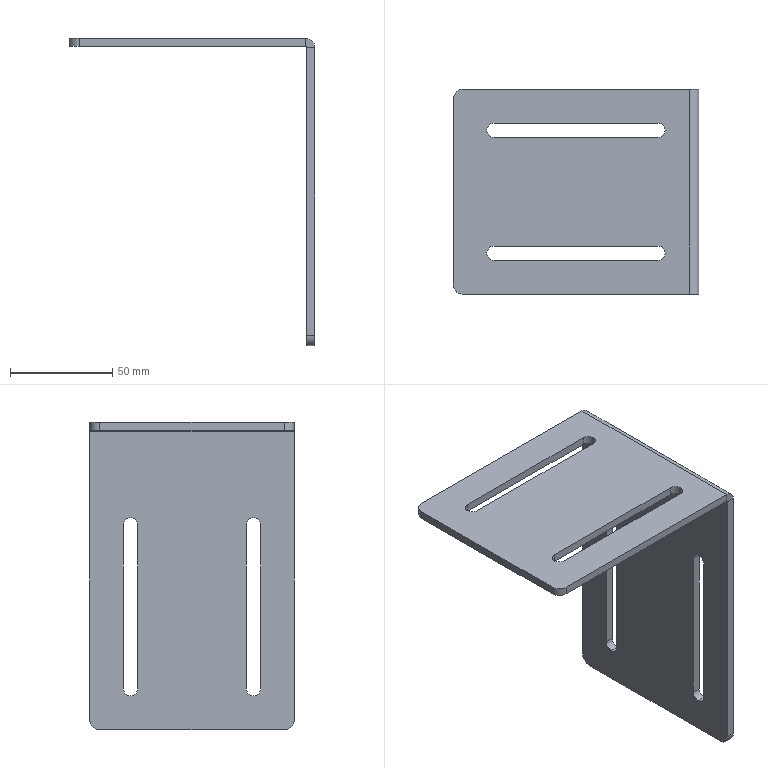Part | SolidWorks | features ICE 2, EdgeFlange 1, Fillet 1, FlatPattern 1, SMBaseFlange 1, SheetMetal 1 | 1 solid | 38 faces | box 120 x 100 x 150 mm | volume 96309 mm3 | plane 20 | cylinder 18 | commonest cylinder face diameters 7 x12 10 x4 1 x1 9 x1
STEP:
#1=CARTESIAN_POINT('',(56.,33.5,-130.));
#2=VERTEX_POINT('',#1);
#3=CARTESIAN_POINT('',(56.,30.,-133.5));
#4=VERTEX_POINT('',#3);
#5=CARTESIAN_POINT('',(56.,30.,-130.));
#6=DIRECTION('',(-1.,0.,0.));
#7=DIRECTION('',(0.,0.,-1.));
#8=AXIS2_PLACEMENT_3D('',#5,#6,#7);
#9=CIRCLE('',#8,3.5);
#10=EDGE_CURVE('',#2,#4,#9,.T.);
#11=ORIENTED_EDGE('',*,*,#10,.T.);
#12=CARTESIAN_POINT('',(60.,30.,-133.5));
#13=VERTEX_POINT('',#12);
#14=CARTESIAN_POINT('',(-60.,30.,-133.5));
#15=DIRECTION('',(1.,0.,0.));
#16=VECTOR('',#15,1000.);
#17=LINE('',#14,#16);
#18=EDGE_CURVE('',#4,#13,#17,.T.);
#19=ORIENTED_EDGE('',*,*,#18,.T.);
#20=CARTESIAN_POINT('',(60.,33.5,-130.));
#21=VERTEX_POINT('',#20);
#22=CARTESIAN_POINT('',(60.,30.,-130.));
#23=DIRECTION('',(-1.,0.,0.));
#24=DIRECTION('',(0.,0.,-1.));
#25=AXIS2_PLACEMENT_3D('',#22,#23,#24);
#26=CIRCLE('',#25,3.5);
#27=EDGE_CURVE('',#21,#13,#26,.T.);
#28=ORIENTED_EDGE('',*,*,#27,.F.);
#29=CARTESIAN_POINT('',(-60.,33.5,-130.));
#30=DIRECTION('',(1.,0.,0.));
#31=VECTOR('',#30,1000.);
#32=LINE('',#29,#31);
#33=EDGE_CURVE('',#2,#21,#32,.T.);
#34=ORIENTED_EDGE('',*,*,#33,.F.);
#35=EDGE_LOOP('',(#11,#19,#28,#34));
#36=FACE_OUTER_BOUND('',#35,.T.);
#37=CARTESIAN_POINT('',(-60.,30.,-130.));
#38=DIRECTION('',(1.,0.,0.));
#39=DIRECTION('',(0.,0.,-1.));
#40=AXIS2_PLACEMENT_3D('',#37,#38,#39);
#41=CYLINDRICAL_SURFACE('',#40,3.5);
#42=ADVANCED_FACE('',(#36),#41,.F.);
#43=CARTESIAN_POINT('',(56.,-26.5,-130.));
#44=VERTEX_POINT('',#43);
#45=CARTESIAN_POINT('',(56.,-30.,-133.5));
#46=VERTEX_POINT('',#45);
#47=CARTESIAN_POINT('',(56.,-30.,-130.));
#48=DIRECTION('',(-1.,0.,0.));
#49=DIRECTION('',(0.,0.,-1.));
#50=AXIS2_PLACEMENT_3D('',#47,#48,#49);
#51=CIRCLE('',#50,3.5);
#52=EDGE_CURVE('',#44,#46,#51,.T.);
#53=ORIENTED_EDGE('',*,*,#52,.T.);
#54=CARTESIAN_POINT('',(60.,-30.,-133.5));
#55=VERTEX_POINT('',#54);
#56=CARTESIAN_POINT('',(-60.,-30.,-133.5));
#57=DIRECTION('',(1.,0.,0.));
#58=VECTOR('',#57,1000.);
#59=LINE('',#56,#58);
#60=EDGE_CURVE('',#46,#55,#59,.T.);
#61=ORIENTED_EDGE('',*,*,#60,.T.);
#62=CARTESIAN_POINT('',(60.,-26.5,-130.));
#63=VERTEX_POINT('',#62);
#64=CARTESIAN_POINT('',(60.,-30.,-130.));
#65=DIRECTION('',(-1.,0.,0.));
#66=DIRECTION('',(0.,0.,-1.));
#67=AXIS2_PLACEMENT_3D('',#64,#65,#66);
#68=CIRCLE('',#67,3.5);
#69=EDGE_CURVE('',#63,#55,#68,.T.);
#70=ORIENTED_EDGE('',*,*,#69,.F.);
#71=CARTESIAN_POINT('',(-60.,-26.5,-130.));
#72=DIRECTION('',(1.,0.,0.));
#73=VECTOR('',#72,1000.);
#74=LINE('',#71,#73);
#75=EDGE_CURVE('',#44,#63,#74,.T.);
#76=ORIENTED_EDGE('',*,*,#75,.F.);
#77=EDGE_LOOP('',(#53,#61,#70,#76));
#78=FACE_OUTER_BOUND('',#77,.T.);
#79=CARTESIAN_POINT('',(-60.,-30.,-130.));
#80=DIRECTION('',(1.,0.,0.));
#81=DIRECTION('',(0.,0.,-1.));
#82=AXIS2_PLACEMENT_3D('',#79,#80,#81);
#83=CYLINDRICAL_SURFACE('',#82,3.5);
#84=ADVANCED_FACE('',(#78),#83,.F.);
#85=CARTESIAN_POINT('',(40.,33.5,-4.));
#86=VERTEX_POINT('',#85);
#87=CARTESIAN_POINT('',(43.5,30.,-4.));
#88=VERTEX_POINT('',#87);
#89=CARTESIAN_POINT('',(40.,30.,-4.));
#90=DIRECTION('',(0.,0.,-1.));
#91=DIRECTION('',(1.,0.,0.));
#92=AXIS2_PLACEMENT_3D('',#89,#90,#91);
#93=CIRCLE('',#92,3.5);
#94=EDGE_CURVE('',#86,#88,#93,.T.);
#95=ORIENTED_EDGE('',*,*,#94,.T.);
#96=CARTESIAN_POINT('',(43.5,30.,0.));
#97=VERTEX_POINT('',#96);
#98=CARTESIAN_POINT('',(43.5,30.,-150.001));
#99=DIRECTION('',(0.,0.,1.));
#100=VECTOR('',#99,1000.);
#101=LINE('',#98,#100);
#102=EDGE_CURVE('',#88,#97,#101,.T.);
#103=ORIENTED_EDGE('',*,*,#102,.T.);
#104=CARTESIAN_POINT('',(40.,33.5,0.));
#105=VERTEX_POINT('',#104);
#106=CARTESIAN_POINT('',(40.,30.,0.));
#107=DIRECTION('',(0.,0.,1.));
#108=DIRECTION('',(1.,0.,0.));
#109=AXIS2_PLACEMENT_3D('',#106,#107,#108);
#110=CIRCLE('',#109,3.5);
#111=EDGE_CURVE('',#97,#105,#110,.T.);
#112=ORIENTED_EDGE('',*,*,#111,.T.);
#113=CARTESIAN_POINT('',(40.,33.5,-150.001));
#114=DIRECTION('',(0.,0.,1.));
#115=VECTOR('',#114,1000.);
#116=LINE('',#113,#115);
#117=EDGE_CURVE('',#86,#105,#116,.T.);
#118=ORIENTED_EDGE('',*,*,#117,.F.);
#119=EDGE_LOOP('',(#95,#103,#112,#118));
#120=FACE_OUTER_BOUND('',#119,.T.);
#121=CARTESIAN_POINT('',(40.,30.,-150.001));
#122=DIRECTION('',(0.,0.,1.));
#123=DIRECTION('',(1.,0.,0.));
#124=AXIS2_PLACEMENT_3D('',#121,#122,#123);
#125=CYLINDRICAL_SURFACE('',#124,3.5);
#126=ADVANCED_FACE('',(#120),#125,.F.);
#127=CARTESIAN_POINT('',(40.,-26.5,-4.));
#128=VERTEX_POINT('',#127);
#129=CARTESIAN_POINT('',(43.5,-30.,-4.));
#130=VERTEX_POINT('',#129);
#131=CARTESIAN_POINT('',(40.,-30.,-4.));
#132=DIRECTION('',(0.,0.,-1.));
#133=DIRECTION('',(1.,0.,0.));
#134=AXIS2_PLACEMENT_3D('',#131,#132,#133);
#135=CIRCLE('',#134,3.5);
#136=EDGE_CURVE('',#128,#130,#135,.T.);
#137=ORIENTED_EDGE('',*,*,#136,.T.);
#138=CARTESIAN_POINT('',(43.5,-30.,0.));
#139=VERTEX_POINT('',#138);
#140=CARTESIAN_POINT('',(43.5,-30.,-150.001));
#141=DIRECTION('',(0.,0.,1.));
#142=VECTOR('',#141,1000.);
#143=LINE('',#140,#142);
#144=EDGE_CURVE('',#130,#139,#143,.T.);
#145=ORIENTED_EDGE('',*,*,#144,.T.);
#146=CARTESIAN_POINT('',(40.,-26.5,0.));
#147=VERTEX_POINT('',#146);
#148=CARTESIAN_POINT('',(40.,-30.,0.));
#149=DIRECTION('',(0.,0.,1.));
#150=DIRECTION('',(1.,0.,0.));
#151=AXIS2_PLACEMENT_3D('',#148,#149,#150);
#152=CIRCLE('',#151,3.5);
#153=EDGE_CURVE('',#139,#147,#152,.T.);
#154=ORIENTED_EDGE('',*,*,#153,.T.);
#155=CARTESIAN_POINT('',(40.,-26.5,-150.001));
#156=DIRECTION('',(0.,0.,1.));
#157=VECTOR('',#156,1000.);
#158=LINE('',#155,#157);
#159=EDGE_CURVE('',#128,#147,#158,.T.);
#160=ORIENTED_EDGE('',*,*,#159,.F.);
#161=EDGE_LOOP('',(#137,#145,#154,#160));
#162=FACE_OUTER_BOUND('',#161,.T.);
#163=CARTESIAN_POINT('',(40.,-30.,-150.001));
#164=DIRECTION('',(0.,0.,1.));
#165=DIRECTION('',(1.,0.,0.));
#166=AXIS2_PLACEMENT_3D('',#163,#164,#165);
#167=CYLINDRICAL_SURFACE('',#166,3.5);
#168=ADVANCED_FACE('',(#162),#167,.F.);
#169=CARTESIAN_POINT('',(60.,-50.,-145.));
#170=VERTEX_POINT('',#169);
#171=CARTESIAN_POINT('',(60.,-50.,-4.5));
#172=VERTEX_POINT('',#171);
#173=CARTESIAN_POINT('',(60.,-50.,-4.));
#174=DIRECTION('',(0.,0.,1.));
#175=VECTOR('',#174,1000.);
#176=LINE('',#173,#175);
#177=EDGE_CURVE('',#170,#172,#176,.T.);
#178=ORIENTED_EDGE('',*,*,#177,.F.);
#179=CARTESIAN_POINT('',(60.,-45.,-150.));
#180=VERTEX_POINT('',#179);
#181=CARTESIAN_POINT('',(60.,-45.,-145.));
#182=DIRECTION('',(1.,0.,0.));
#183=DIRECTION('',(0.,0.,-1.));
#184=AXIS2_PLACEMENT_3D('',#181,#182,#183);
#185=CIRCLE('',#184,5.);
#186=EDGE_CURVE('',#170,#180,#185,.T.);
#187=ORIENTED_EDGE('',*,*,#186,.T.);
#188=CARTESIAN_POINT('',(60.,45.,-150.));
#189=VERTEX_POINT('',#188);
#190=CARTESIAN_POINT('',(60.,-50.,-150.));
#191=DIRECTION('',(0.,-1.,0.));
#192=VECTOR('',#191,1000.);
#193=LINE('',#190,#192);
#194=EDGE_CURVE('',#189,#180,#193,.T.);
#195=ORIENTED_EDGE('',*,*,#194,.F.);
#196=CARTESIAN_POINT('',(60.,50.,-145.));
#197=VERTEX_POINT('',#196);
#198=CARTESIAN_POINT('',(60.,45.,-145.));
#199=DIRECTION('',(1.,0.,0.));
#200=DIRECTION('',(0.,0.,-1.));
#201=AXIS2_PLACEMENT_3D('',#198,#199,#200);
#202=CIRCLE('',#201,5.);
#203=EDGE_CURVE('',#189,#197,#202,.T.);
#204=ORIENTED_EDGE('',*,*,#203,.T.);
#205=CARTESIAN_POINT('',(60.,50.,-4.5));
#206=VERTEX_POINT('',#205);
#207=CARTESIAN_POINT('',(60.,50.,-150.));
#208=DIRECTION('',(0.,0.,-1.));
#209=VECTOR('',#208,1000.);
#210=LINE('',#207,#209);
#211=EDGE_CURVE('',#206,#197,#210,.T.);
#212=ORIENTED_EDGE('',*,*,#211,.F.);
#213=CARTESIAN_POINT('',(60.,0.,-4.5));
#214=DIRECTION('',(0.,-1.,0.));
#215=VECTOR('',#214,1000.);
#216=LINE('',#213,#215);
#217=EDGE_CURVE('',#206,#172,#216,.T.);
#218=ORIENTED_EDGE('',*,*,#217,.T.);
#219=EDGE_LOOP('',(#178,#187,#195,#204,#212,#218));
#220=FACE_OUTER_BOUND('',#219,.T.);
#221=CARTESIAN_POINT('',(60.,-26.5,-50.));
#222=VERTEX_POINT('',#221);
#223=CARTESIAN_POINT('',(60.,-26.5,-130.));
#224=DIRECTION('',(0.,0.,-1.));
#225=VECTOR('',#224,1000.);
#226=LINE('',#223,#225);
#227=EDGE_CURVE('',#222,#63,#226,.T.);
#228=ORIENTED_EDGE('',*,*,#227,.T.);
#229=ORIENTED_EDGE('',*,*,#69,.T.);
#230=CARTESIAN_POINT('',(60.,-33.5,-130.));
#231=VERTEX_POINT('',#230);
#232=CARTESIAN_POINT('',(60.,-30.,-130.));
#233=DIRECTION('',(-1.,0.,0.));
#234=DIRECTION('',(0.,0.,-1.));
#235=AXIS2_PLACEMENT_3D('',#232,#233,#234);
#236=CIRCLE('',#235,3.5);
#237=EDGE_CURVE('',#55,#231,#236,.T.);
#238=ORIENTED_EDGE('',*,*,#237,.T.);
#239=CARTESIAN_POINT('',(60.,-33.5,-50.));
#240=VERTEX_POINT('',#239);
#241=CARTESIAN_POINT('',(60.,-33.5,-130.));
#242=DIRECTION('',(0.,0.,1.));
#243=VECTOR('',#242,1000.);
#244=LINE('',#241,#243);
#245=EDGE_CURVE('',#231,#240,#244,.T.);
#246=ORIENTED_EDGE('',*,*,#245,.T.);
#247=CARTESIAN_POINT('',(60.,-30.,-50.));
#248=DIRECTION('',(-1.,0.,0.));
#249=DIRECTION('',(0.,0.,-1.));
#250=AXIS2_PLACEMENT_3D('',#247,#248,#249);
#251=CIRCLE('',#250,3.5);
#252=EDGE_CURVE('',#240,#222,#251,.T.);
#253=ORIENTED_EDGE('',*,*,#252,.T.);
#254=EDGE_LOOP('',(#228,#229,#238,#246,#253));
#255=FACE_BOUND('',#254,.T.);
#256=CARTESIAN_POINT('',(60.,33.5,-50.));
#257=VERTEX_POINT('',#256);
#258=CARTESIAN_POINT('',(60.,33.5,-130.));
#259=DIRECTION('',(0.,0.,-1.));
#260=VECTOR('',#259,1000.);
#261=LINE('',#258,#260);
#262=EDGE_CURVE('',#257,#21,#261,.T.);
#263=ORIENTED_EDGE('',*,*,#262,.T.);
#264=ORIENTED_EDGE('',*,*,#27,.T.);
#265=CARTESIAN_POINT('',(60.,26.5,-130.));
#266=VERTEX_POINT('',#265);
#267=CARTESIAN_POINT('',(60.,30.,-130.));
#268=DIRECTION('',(-1.,0.,0.));
#269=DIRECTION('',(0.,0.,-1.));
#270=AXIS2_PLACEMENT_3D('',#267,#268,#269);
#271=CIRCLE('',#270,3.5);
#272=EDGE_CURVE('',#13,#266,#271,.T.);
#273=ORIENTED_EDGE('',*,*,#272,.T.);
#274=CARTESIAN_POINT('',(60.,26.5,-50.));
#275=VERTEX_POINT('',#274);
#276=CARTESIAN_POINT('',(60.,26.5,-130.));
#277=DIRECTION('',(0.,0.,1.));
#278=VECTOR('',#277,1000.);
#279=LINE('',#276,#278);
#280=EDGE_CURVE('',#266,#275,#279,.T.);
#281=ORIENTED_EDGE('',*,*,#280,.T.);
#282=CARTESIAN_POINT('',(60.,30.,-50.));
#283=DIRECTION('',(-1.,0.,0.));
#284=DIRECTION('',(0.,0.,-1.));
#285=AXIS2_PLACEMENT_3D('',#282,#283,#284);
#286=CIRCLE('',#285,3.5);
#287=EDGE_CURVE('',#275,#257,#286,.T.);
#288=ORIENTED_EDGE('',*,*,#287,.T.);
#289=EDGE_LOOP('',(#263,#264,#273,#281,#288));
#290=FACE_BOUND('',#289,.T.);
#291=CARTESIAN_POINT('',(60.,0.,0.));
#292=DIRECTION('',(1.,0.,0.));
#293=DIRECTION('',(0.,0.,-1.));
#294=AXIS2_PLACEMENT_3D('',#291,#292,#293);
#295=PLANE('',#294);
#296=ADVANCED_FACE('',(#220,#255,#290),#295,.T.);
#297=ORIENTED_EDGE('',*,*,#52,.F.);
#298=CARTESIAN_POINT('',(56.,-26.5,-50.));
#299=VERTEX_POINT('',#298);
#300=CARTESIAN_POINT('',(56.,-26.5,0.));
#301=DIRECTION('',(0.,0.,-1.));
#302=VECTOR('',#301,1000.);
#303=LINE('',#300,#302);
#304=EDGE_CURVE('',#299,#44,#303,.T.);
#305=ORIENTED_EDGE('',*,*,#304,.F.);
#306=CARTESIAN_POINT('',(56.,-33.5,-50.));
#307=VERTEX_POINT('',#306);
#308=CARTESIAN_POINT('',(56.,-30.,-50.));
#309=DIRECTION('',(-1.,0.,0.));
#310=DIRECTION('',(0.,0.,-1.));
#311=AXIS2_PLACEMENT_3D('',#308,#309,#310);
#312=CIRCLE('',#311,3.5);
#313=EDGE_CURVE('',#307,#299,#312,.T.);
#314=ORIENTED_EDGE('',*,*,#313,.F.);
#315=CARTESIAN_POINT('',(56.,-33.5,-130.));
#316=VERTEX_POINT('',#315);
#317=CARTESIAN_POINT('',(56.,-33.5,0.));
#318=DIRECTION('',(0.,0.,1.));
#319=VECTOR('',#318,1000.);
#320=LINE('',#317,#319);
#321=EDGE_CURVE('',#316,#307,#320,.T.);
#322=ORIENTED_EDGE('',*,*,#321,.F.);
#323=CARTESIAN_POINT('',(56.,-30.,-130.));
#324=DIRECTION('',(-1.,0.,0.));
#325=DIRECTION('',(0.,0.,-1.));
#326=AXIS2_PLACEMENT_3D('',#323,#324,#325);
#327=CIRCLE('',#326,3.5);
#328=EDGE_CURVE('',#46,#316,#327,.T.);
#329=ORIENTED_EDGE('',*,*,#328,.F.);
#330=EDGE_LOOP('',(#297,#305,#314,#322,#329));
#331=FACE_BOUND('',#330,.T.);
#332=CARTESIAN_POINT('',(56.,45.,-150.));
#333=VERTEX_POINT('',#332);
#334=CARTESIAN_POINT('',(56.,-45.,-150.));
#335=VERTEX_POINT('',#334);
#336=CARTESIAN_POINT('',(56.,0.,-150.));
#337=DIRECTION('',(0.,-1.,0.));
#338=VECTOR('',#337,1000.);
#339=LINE('',#336,#338);
#340=EDGE_CURVE('',#333,#335,#339,.T.);
#341=ORIENTED_EDGE('',*,*,#340,.T.);
#342=CARTESIAN_POINT('',(56.,-50.,-145.));
#343=VERTEX_POINT('',#342);
#344=CARTESIAN_POINT('',(56.,-45.,-145.));
#345=DIRECTION('',(-1.,0.,0.));
#346=DIRECTION('',(0.,0.,-1.));
#347=AXIS2_PLACEMENT_3D('',#344,#345,#346);
#348=CIRCLE('',#347,5.);
#349=EDGE_CURVE('',#335,#343,#348,.T.);
#350=ORIENTED_EDGE('',*,*,#349,.T.);
#351=CARTESIAN_POINT('',(56.,-50.,-4.5));
#352=VERTEX_POINT('',#351);
#353=CARTESIAN_POINT('',(56.,-50.,0.));
#354=DIRECTION('',(0.,0.,1.));
#355=VECTOR('',#354,1000.);
#356=LINE('',#353,#355);
#357=EDGE_CURVE('',#343,#352,#356,.T.);
#358=ORIENTED_EDGE('',*,*,#357,.T.);
#359=CARTESIAN_POINT('',(56.,50.,-4.5));
#360=VERTEX_POINT('',#359);
#361=CARTESIAN_POINT('',(56.,50.,-4.5));
#362=DIRECTION('',(0.,-1.,0.));
#363=VECTOR('',#362,1000.);
#364=LINE('',#361,#363);
#365=EDGE_CURVE('',#360,#352,#364,.T.);
#366=ORIENTED_EDGE('',*,*,#365,.F.);
#367=CARTESIAN_POINT('',(56.,50.,-145.));
#368=VERTEX_POINT('',#367);
#369=CARTESIAN_POINT('',(56.,50.,0.));
#370=DIRECTION('',(0.,0.,-1.));
#371=VECTOR('',#370,1000.);
#372=LINE('',#369,#371);
#373=EDGE_CURVE('',#360,#368,#372,.T.);
#374=ORIENTED_EDGE('',*,*,#373,.T.);
#375=CARTESIAN_POINT('',(56.,45.,-145.));
#376=DIRECTION('',(-1.,0.,0.));
#377=DIRECTION('',(0.,0.,-1.));
#378=AXIS2_PLACEMENT_3D('',#375,#376,#377);
#379=CIRCLE('',#378,5.);
#380=EDGE_CURVE('',#368,#333,#379,.T.);
#381=ORIENTED_EDGE('',*,*,#380,.T.);
#382=EDGE_LOOP('',(#341,#350,#358,#366,#374,#381));
#383=FACE_OUTER_BOUND('',#382,.T.);
#384=ORIENTED_EDGE('',*,*,#10,.F.);
#385=CARTESIAN_POINT('',(56.,33.5,-50.));
#386=VERTEX_POINT('',#385);
#387=CARTESIAN_POINT('',(56.,33.5,0.));
#388=DIRECTION('',(0.,0.,-1.));
#389=VECTOR('',#388,1000.);
#390=LINE('',#387,#389);
#391=EDGE_CURVE('',#386,#2,#390,.T.);
#392=ORIENTED_EDGE('',*,*,#391,.F.);
#393=CARTESIAN_POINT('',(56.,26.5,-50.));
#394=VERTEX_POINT('',#393);
#395=CARTESIAN_POINT('',(56.,30.,-50.));
#396=DIRECTION('',(-1.,0.,0.));
#397=DIRECTION('',(0.,0.,-1.));
#398=AXIS2_PLACEMENT_3D('',#395,#396,#397);
#399=CIRCLE('',#398,3.5);
#400=EDGE_CURVE('',#394,#386,#399,.T.);
#401=ORIENTED_EDGE('',*,*,#400,.F.);
#402=CARTESIAN_POINT('',(56.,26.5,-130.));
#403=VERTEX_POINT('',#402);
#404=CARTESIAN_POINT('',(56.,26.5,0.));
#405=DIRECTION('',(0.,0.,1.));
#406=VECTOR('',#405,1000.);
#407=LINE('',#404,#406);
#408=EDGE_CURVE('',#403,#394,#407,.T.);
#409=ORIENTED_EDGE('',*,*,#408,.F.);
#410=CARTESIAN_POINT('',(56.,30.,-130.));
#411=DIRECTION('',(-1.,0.,0.));
#412=DIRECTION('',(0.,0.,-1.));
#413=AXIS2_PLACEMENT_3D('',#410,#411,#412);
#414=CIRCLE('',#413,3.5);
#415=EDGE_CURVE('',#4,#403,#414,.T.);
#416=ORIENTED_EDGE('',*,*,#415,.F.);
#417=EDGE_LOOP('',(#384,#392,#401,#409,#416));
#418=FACE_BOUND('',#417,.T.);
#419=CARTESIAN_POINT('',(56.,0.,0.));
#420=DIRECTION('',(1.,0.,0.));
#421=DIRECTION('',(0.,0.,-1.));
#422=AXIS2_PLACEMENT_3D('',#419,#420,#421);
#423=PLANE('',#422);
#424=ADVANCED_FACE('',(#331,#383,#418),#423,.F.);
#425=CARTESIAN_POINT('',(-55.,-50.,0.));
#426=VERTEX_POINT('',#425);
#427=CARTESIAN_POINT('',(55.5,-50.,0.));
#428=VERTEX_POINT('',#427);
#429=CARTESIAN_POINT('',(60.,-50.,0.));
#430=DIRECTION('',(1.,0.,0.));
#431=VECTOR('',#430,1000.);
#432=LINE('',#429,#431);
#433=EDGE_CURVE('',#426,#428,#432,.T.);
#434=ORIENTED_EDGE('',*,*,#433,.F.);
#435=CARTESIAN_POINT('',(-55.,-50.,-4.));
#436=VERTEX_POINT('',#435);
#437=CARTESIAN_POINT('',(-55.,-50.,-4.));
#438=DIRECTION('',(0.,0.,-1.));
#439=VECTOR('',#438,1000.);
#440=LINE('',#437,#439);
#441=EDGE_CURVE('',#426,#436,#440,.T.);
#442=ORIENTED_EDGE('',*,*,#441,.T.);
#443=CARTESIAN_POINT('',(55.5,-50.,-4.));
#444=VERTEX_POINT('',#443);
#445=CARTESIAN_POINT('',(60.,-50.,-4.));
#446=DIRECTION('',(1.,0.,0.));
#447=VECTOR('',#446,1000.);
#448=LINE('',#445,#447);
#449=EDGE_CURVE('',#436,#444,#448,.T.);
#450=ORIENTED_EDGE('',*,*,#449,.T.);
#451=CARTESIAN_POINT('',(55.5,-50.,-4.));
#452=DIRECTION('',(0.,0.,1.));
#453=VECTOR('',#452,1000.);
#454=LINE('',#451,#453);
#455=EDGE_CURVE('',#444,#428,#454,.T.);
#456=ORIENTED_EDGE('',*,*,#455,.T.);
#457=EDGE_LOOP('',(#434,#442,#450,#456));
#458=FACE_OUTER_BOUND('',#457,.T.);
#459=CARTESIAN_POINT('',(60.,-50.,-4.));
#460=DIRECTION('',(0.,-1.,0.));
#461=DIRECTION('',(1.,0.,0.));
#462=AXIS2_PLACEMENT_3D('',#459,#460,#461);
#463=PLANE('',#462);
#464=ADVANCED_FACE('',(#458),#463,.T.);
#465=CARTESIAN_POINT('',(-40.,33.5,-4.));
#466=VERTEX_POINT('',#465);
#467=CARTESIAN_POINT('',(-40.,33.5,-4.));
#468=DIRECTION('',(1.,0.,0.));
#469=VECTOR('',#468,1000.);
#470=LINE('',#467,#469);
#471=EDGE_CURVE('',#466,#86,#470,.T.);
#472=ORIENTED_EDGE('',*,*,#471,.F.);
#473=CARTESIAN_POINT('',(-40.,26.5,-4.));
#474=VERTEX_POINT('',#473);
#475=CARTESIAN_POINT('',(-40.,30.,-4.));
#476=DIRECTION('',(0.,0.,-1.));
#477=DIRECTION('',(1.,0.,0.));
#478=AXIS2_PLACEMENT_3D('',#475,#476,#477);
#479=CIRCLE('',#478,3.5);
#480=EDGE_CURVE('',#474,#466,#479,.T.);
#481=ORIENTED_EDGE('',*,*,#480,.F.);
#482=CARTESIAN_POINT('',(40.,26.5,-4.));
#483=VERTEX_POINT('',#482);
#484=CARTESIAN_POINT('',(-40.,26.5,-4.));
#485=DIRECTION('',(-1.,0.,0.));
#486=VECTOR('',#485,1000.);
#487=LINE('',#484,#486);
#488=EDGE_CURVE('',#483,#474,#487,.T.);
#489=ORIENTED_EDGE('',*,*,#488,.F.);
#490=CARTESIAN_POINT('',(40.,30.,-4.));
#491=DIRECTION('',(0.,0.,-1.));
#492=DIRECTION('',(1.,0.,0.));
#493=AXIS2_PLACEMENT_3D('',#490,#491,#492);
#494=CIRCLE('',#493,3.5);
#495=EDGE_CURVE('',#88,#483,#494,.T.);
#496=ORIENTED_EDGE('',*,*,#495,.F.);
#497=ORIENTED_EDGE('',*,*,#94,.F.);
#498=EDGE_LOOP('',(#472,#481,#489,#496,#497));
#499=FACE_BOUND('',#498,.T.);
#500=CARTESIAN_POINT('',(-40.,-26.5,-4.));
#501=VERTEX_POINT('',#500);
#502=CARTESIAN_POINT('',(-40.,-26.5,-4.));
#503=DIRECTION('',(1.,0.,0.));
#504=VECTOR('',#503,1000.);
#505=LINE('',#502,#504);
#506=EDGE_CURVE('',#501,#128,#505,.T.);
#507=ORIENTED_EDGE('',*,*,#506,.F.);
#508=CARTESIAN_POINT('',(-40.,-33.5,-4.));
#509=VERTEX_POINT('',#508);
#510=CARTESIAN_POINT('',(-40.,-30.,-4.));
#511=DIRECTION('',(0.,0.,-1.));
#512=DIRECTION('',(1.,0.,0.));
#513=AXIS2_PLACEMENT_3D('',#510,#511,#512);
#514=CIRCLE('',#513,3.5);
#515=EDGE_CURVE('',#509,#501,#514,.T.);
#516=ORIENTED_EDGE('',*,*,#515,.F.);
#517=CARTESIAN_POINT('',(40.,-33.5,-4.));
#518=VERTEX_POINT('',#517);
#519=CARTESIAN_POINT('',(-40.,-33.5,-4.));
#520=DIRECTION('',(-1.,0.,0.));
#521=VECTOR('',#520,1000.);
#522=LINE('',#519,#521);
#523=EDGE_CURVE('',#518,#509,#522,.T.);
#524=ORIENTED_EDGE('',*,*,#523,.F.);
#525=CARTESIAN_POINT('',(40.,-30.,-4.));
#526=DIRECTION('',(0.,0.,-1.));
#527=DIRECTION('',(1.,0.,0.));
#528=AXIS2_PLACEMENT_3D('',#525,#526,#527);
#529=CIRCLE('',#528,3.5);
#530=EDGE_CURVE('',#130,#518,#529,.T.);
#531=ORIENTED_EDGE('',*,*,#530,.F.);
#532=ORIENTED_EDGE('',*,*,#136,.F.);
#533=EDGE_LOOP('',(#507,#516,#524,#531,#532));
#534=FACE_BOUND('',#533,.T.);
#535=ORIENTED_EDGE('',*,*,#449,.F.);
#536=CARTESIAN_POINT('',(-60.,-45.,-4.));
#537=VERTEX_POINT('',#536);
#538=CARTESIAN_POINT('',(-55.,-45.,-4.));
#539=DIRECTION('',(0.,0.,-1.));
#540=DIRECTION('',(1.,0.,0.));
#541=AXIS2_PLACEMENT_3D('',#538,#539,#540);
#542=CIRCLE('',#541,5.);
#543=EDGE_CURVE('',#436,#537,#542,.T.);
#544=ORIENTED_EDGE('',*,*,#543,.T.);
#545=CARTESIAN_POINT('',(-60.,45.,-4.));
#546=VERTEX_POINT('',#545);
#547=CARTESIAN_POINT('',(-60.,-50.,-4.));
#548=DIRECTION('',(0.,-1.,0.));
#549=VECTOR('',#548,1000.);
#550=LINE('',#547,#549);
#551=EDGE_CURVE('',#546,#537,#550,.T.);
#552=ORIENTED_EDGE('',*,*,#551,.F.);
#553=CARTESIAN_POINT('',(-55.,50.,-4.));
#554=VERTEX_POINT('',#553);
#555=CARTESIAN_POINT('',(-55.,45.,-4.));
#556=DIRECTION('',(0.,0.,-1.));
#557=DIRECTION('',(1.,0.,0.));
#558=AXIS2_PLACEMENT_3D('',#555,#556,#557);
#559=CIRCLE('',#558,5.);
#560=EDGE_CURVE('',#546,#554,#559,.T.);
#561=ORIENTED_EDGE('',*,*,#560,.T.);
#562=CARTESIAN_POINT('',(55.5,50.,-4.));
#563=VERTEX_POINT('',#562);
#564=CARTESIAN_POINT('',(60.,50.,-4.));
#565=DIRECTION('',(-1.,0.,0.));
#566=VECTOR('',#565,1000.);
#567=LINE('',#564,#566);
#568=EDGE_CURVE('',#563,#554,#567,.T.);
#569=ORIENTED_EDGE('',*,*,#568,.F.);
#570=CARTESIAN_POINT('',(55.5,-50.,-4.));
#571=DIRECTION('',(0.,1.,0.));
#572=VECTOR('',#571,1000.);
#573=LINE('',#570,#572);
#574=EDGE_CURVE('',#444,#563,#573,.T.);
#575=ORIENTED_EDGE('',*,*,#574,.F.);
#576=EDGE_LOOP('',(#535,#544,#552,#561,#569,#575));
#577=FACE_OUTER_BOUND('',#576,.T.);
#578=CARTESIAN_POINT('',(0.,0.,-4.));
#579=DIRECTION('',(0.,0.,1.));
#580=DIRECTION('',(1.,0.,0.));
#581=AXIS2_PLACEMENT_3D('',#578,#579,#580);
#582=PLANE('',#581);
#583=ADVANCED_FACE('',(#499,#534,#577),#582,.F.);
#584=CARTESIAN_POINT('',(-40.,33.5,0.));
#585=VERTEX_POINT('',#584);
#586=CARTESIAN_POINT('',(-40.,26.5,0.));
#587=VERTEX_POINT('',#586);
#588=CARTESIAN_POINT('',(-40.,30.,0.));
#589=DIRECTION('',(0.,0.,1.));
#590=DIRECTION('',(1.,0.,0.));
#591=AXIS2_PLACEMENT_3D('',#588,#589,#590);
#592=CIRCLE('',#591,3.5);
#593=EDGE_CURVE('',#585,#587,#592,.T.);
#594=ORIENTED_EDGE('',*,*,#593,.F.);
#595=CARTESIAN_POINT('',(-40.,33.5,0.));
#596=DIRECTION('',(-1.,0.,0.));
#597=VECTOR('',#596,1000.);
#598=LINE('',#595,#597);
#599=EDGE_CURVE('',#105,#585,#598,.T.);
#600=ORIENTED_EDGE('',*,*,#599,.F.);
#601=ORIENTED_EDGE('',*,*,#111,.F.);
#602=CARTESIAN_POINT('',(40.,26.5,0.));
#603=VERTEX_POINT('',#602);
#604=CARTESIAN_POINT('',(40.,30.,0.));
#605=DIRECTION('',(0.,0.,1.));
#606=DIRECTION('',(1.,0.,0.));
#607=AXIS2_PLACEMENT_3D('',#604,#605,#606);
#608=CIRCLE('',#607,3.5);
#609=EDGE_CURVE('',#603,#97,#608,.T.);
#610=ORIENTED_EDGE('',*,*,#609,.F.);
#611=CARTESIAN_POINT('',(-40.,26.5,0.));
#612=DIRECTION('',(1.,0.,0.));
#613=VECTOR('',#612,1000.);
#614=LINE('',#611,#613);
#615=EDGE_CURVE('',#587,#603,#614,.T.);
#616=ORIENTED_EDGE('',*,*,#615,.F.);
#617=EDGE_LOOP('',(#594,#600,#601,#610,#616));
#618=FACE_BOUND('',#617,.T.);
#619=CARTESIAN_POINT('',(-40.,-26.5,0.));
#620=VERTEX_POINT('',#619);
#621=CARTESIAN_POINT('',(-40.,-33.5,0.));
#622=VERTEX_POINT('',#621);
#623=CARTESIAN_POINT('',(-40.,-30.,0.));
#624=DIRECTION('',(0.,0.,1.));
#625=DIRECTION('',(1.,0.,0.));
#626=AXIS2_PLACEMENT_3D('',#623,#624,#625);
#627=CIRCLE('',#626,3.5);
#628=EDGE_CURVE('',#620,#622,#627,.T.);
#629=ORIENTED_EDGE('',*,*,#628,.F.);
#630=CARTESIAN_POINT('',(-40.,-26.5,0.));
#631=DIRECTION('',(-1.,0.,0.));
#632=VECTOR('',#631,1000.);
#633=LINE('',#630,#632);
#634=EDGE_CURVE('',#147,#620,#633,.T.);
#635=ORIENTED_EDGE('',*,*,#634,.F.);
#636=ORIENTED_EDGE('',*,*,#153,.F.);
#637=CARTESIAN_POINT('',(40.,-33.5,0.));
#638=VERTEX_POINT('',#637);
#639=CARTESIAN_POINT('',(40.,-30.,0.));
#640=DIRECTION('',(0.,0.,1.));
#641=DIRECTION('',(1.,0.,0.));
#642=AXIS2_PLACEMENT_3D('',#639,#640,#641);
#643=CIRCLE('',#642,3.5);
#644=EDGE_CURVE('',#638,#139,#643,.T.);
#645=ORIENTED_EDGE('',*,*,#644,.F.);
#646=CARTESIAN_POINT('',(-40.,-33.5,0.));
#647=DIRECTION('',(1.,0.,0.));
#648=VECTOR('',#647,1000.);
#649=LINE('',#646,#648);
#650=EDGE_CURVE('',#622,#638,#649,.T.);
#651=ORIENTED_EDGE('',*,*,#650,.F.);
#652=EDGE_LOOP('',(#629,#635,#636,#645,#651));
#653=FACE_BOUND('',#652,.T.);
#654=CARTESIAN_POINT('',(-60.,45.,0.));
#655=VERTEX_POINT('',#654);
#656=CARTESIAN_POINT('',(-60.,-45.,0.));
#657=VERTEX_POINT('',#656);
#658=CARTESIAN_POINT('',(-60.,-50.,0.));
#659=DIRECTION('',(0.,-1.,0.));
#660=VECTOR('',#659,1000.);
#661=LINE('',#658,#660);
#662=EDGE_CURVE('',#655,#657,#661,.T.);
#663=ORIENTED_EDGE('',*,*,#662,.T.);
#664=CARTESIAN_POINT('',(-55.,-45.,0.));
#665=DIRECTION('',(0.,0.,1.));
#666=DIRECTION('',(1.,0.,0.));
#667=AXIS2_PLACEMENT_3D('',#664,#665,#666);
#668=CIRCLE('',#667,5.);
#669=EDGE_CURVE('',#657,#426,#668,.T.);
#670=ORIENTED_EDGE('',*,*,#669,.T.);
#671=ORIENTED_EDGE('',*,*,#433,.T.);
#672=CARTESIAN_POINT('',(55.5,50.,0.));
#673=VERTEX_POINT('',#672);
#674=CARTESIAN_POINT('',(55.5,-50.,0.));
#675=DIRECTION('',(0.,1.,0.));
#676=VECTOR('',#675,1000.);
#677=LINE('',#674,#676);
#678=EDGE_CURVE('',#428,#673,#677,.T.);
#679=ORIENTED_EDGE('',*,*,#678,.T.);
#680=CARTESIAN_POINT('',(-55.,50.,0.));
#681=VERTEX_POINT('',#680);
#682=CARTESIAN_POINT('',(60.,50.,0.));
#683=DIRECTION('',(-1.,0.,0.));
#684=VECTOR('',#683,1000.);
#685=LINE('',#682,#684);
#686=EDGE_CURVE('',#673,#681,#685,.T.);
#687=ORIENTED_EDGE('',*,*,#686,.T.);
#688=CARTESIAN_POINT('',(-55.,45.,0.));
#689=DIRECTION('',(0.,0.,1.));
#690=DIRECTION('',(1.,0.,0.));
#691=AXIS2_PLACEMENT_3D('',#688,#689,#690);
#692=CIRCLE('',#691,5.);
#693=EDGE_CURVE('',#681,#655,#692,.T.);
#694=ORIENTED_EDGE('',*,*,#693,.T.);
#695=EDGE_LOOP('',(#663,#670,#671,#679,#687,#694));
#696=FACE_OUTER_BOUND('',#695,.T.);
#697=CARTESIAN_POINT('',(0.,0.,0.));
#698=DIRECTION('',(0.,0.,1.));
#699=DIRECTION('',(1.,0.,0.));
#700=AXIS2_PLACEMENT_3D('',#697,#698,#699);
#701=PLANE('',#700);
#702=ADVANCED_FACE('',(#618,#653,#696),#701,.T.);
#703=ORIENTED_EDGE('',*,*,#551,.T.);
#704=CARTESIAN_POINT('',(-60.,-45.,-4.));
#705=DIRECTION('',(0.,0.,1.));
#706=VECTOR('',#705,1000.);
#707=LINE('',#704,#706);
#708=EDGE_CURVE('',#537,#657,#707,.T.);
#709=ORIENTED_EDGE('',*,*,#708,.T.);
#710=ORIENTED_EDGE('',*,*,#662,.F.);
#711=CARTESIAN_POINT('',(-60.,45.,-4.));
#712=DIRECTION('',(0.,0.,-1.));
#713=VECTOR('',#712,1000.);
#714=LINE('',#711,#713);
#715=EDGE_CURVE('',#655,#546,#714,.T.);
#716=ORIENTED_EDGE('',*,*,#715,.T.);
#717=EDGE_LOOP('',(#703,#709,#710,#716));
#718=FACE_OUTER_BOUND('',#717,.T.);
#719=CARTESIAN_POINT('',(-60.,-50.,-4.));
#720=DIRECTION('',(-1.,0.,0.));
#721=DIRECTION('',(0.,0.,1.));
#722=AXIS2_PLACEMENT_3D('',#719,#720,#721);
#723=PLANE('',#722);
#724=ADVANCED_FACE('',(#718),#723,.T.);
#725=ORIENTED_EDGE('',*,*,#568,.T.);
#726=CARTESIAN_POINT('',(-55.,50.,-4.));
#727=DIRECTION('',(0.,0.,1.));
#728=VECTOR('',#727,1000.);
#729=LINE('',#726,#728);
#730=EDGE_CURVE('',#554,#681,#729,.T.);
#731=ORIENTED_EDGE('',*,*,#730,.T.);
#732=ORIENTED_EDGE('',*,*,#686,.F.);
#733=CARTESIAN_POINT('',(55.5,50.,-4.));
#734=DIRECTION('',(0.,0.,1.));
#735=VECTOR('',#734,1000.);
#736=LINE('',#733,#735);
#737=EDGE_CURVE('',#563,#673,#736,.T.);
#738=ORIENTED_EDGE('',*,*,#737,.F.);
#739=EDGE_LOOP('',(#725,#731,#732,#738));
#740=FACE_OUTER_BOUND('',#739,.T.);
#741=CARTESIAN_POINT('',(60.,50.,-4.));
#742=DIRECTION('',(0.,1.,0.));
#743=DIRECTION('',(-1.,0.,0.));
#744=AXIS2_PLACEMENT_3D('',#741,#742,#743);
#745=PLANE('',#744);
#746=ADVANCED_FACE('',(#740),#745,.T.);
#747=CARTESIAN_POINT('',(60.,50.,-4.5));
#748=DIRECTION('',(1.,0.,0.));
#749=VECTOR('',#748,1000.);
#750=LINE('',#747,#749);
#751=EDGE_CURVE('',#360,#206,#750,.T.);
#752=ORIENTED_EDGE('',*,*,#751,.F.);
#753=CARTESIAN_POINT('',(55.5,50.,-4.5));
#754=DIRECTION('',(0.,1.,0.));
#755=DIRECTION('',(0.,0.,-1.));
#756=AXIS2_PLACEMENT_3D('',#753,#754,#755);
#757=CIRCLE('',#756,0.5);
#758=EDGE_CURVE('',#563,#360,#757,.T.);
#759=ORIENTED_EDGE('',*,*,#758,.F.);
#760=ORIENTED_EDGE('',*,*,#737,.T.);
#761=CARTESIAN_POINT('',(55.5,50.,-4.5));
#762=DIRECTION('',(0.,1.,0.));
#763=DIRECTION('',(0.,0.,-1.));
#764=AXIS2_PLACEMENT_3D('',#761,#762,#763);
#765=CIRCLE('',#764,4.5);
#766=EDGE_CURVE('',#673,#206,#765,.T.);
#767=ORIENTED_EDGE('',*,*,#766,.T.);
#768=EDGE_LOOP('',(#752,#759,#760,#767));
#769=FACE_OUTER_BOUND('',#768,.T.);
#770=CARTESIAN_POINT('',(55.5,50.,-4.5));
#771=DIRECTION('',(0.,1.,0.));
#772=DIRECTION('',(0.,0.,1.));
#773=AXIS2_PLACEMENT_3D('',#770,#771,#772);
#774=PLANE('',#773);
#775=ADVANCED_FACE('',(#769),#774,.T.);
#776=CARTESIAN_POINT('',(55.5,-50.,-4.5));
#777=DIRECTION('',(0.,-1.,0.));
#778=DIRECTION('',(0.,0.,-1.));
#779=AXIS2_PLACEMENT_3D('',#776,#777,#778);
#780=CIRCLE('',#779,0.5);
#781=EDGE_CURVE('',#352,#444,#780,.T.);
#782=ORIENTED_EDGE('',*,*,#781,.F.);
#783=CARTESIAN_POINT('',(56.,-50.,-4.5));
#784=DIRECTION('',(1.,0.,0.));
#785=VECTOR('',#784,1000.);
#786=LINE('',#783,#785);
#787=EDGE_CURVE('',#352,#172,#786,.T.);
#788=ORIENTED_EDGE('',*,*,#787,.T.);
#789=CARTESIAN_POINT('',(55.5,-50.,-4.5));
#790=DIRECTION('',(0.,-1.,0.));
#791=DIRECTION('',(0.,0.,-1.));
#792=AXIS2_PLACEMENT_3D('',#789,#790,#791);
#793=CIRCLE('',#792,4.5);
#794=EDGE_CURVE('',#172,#428,#793,.T.);
#795=ORIENTED_EDGE('',*,*,#794,.T.);
#796=ORIENTED_EDGE('',*,*,#455,.F.);
#797=EDGE_LOOP('',(#782,#788,#795,#796));
#798=FACE_OUTER_BOUND('',#797,.T.);
#799=CARTESIAN_POINT('',(55.5,-50.,-4.5));
#800=DIRECTION('',(0.,1.,0.));
#801=DIRECTION('',(0.,0.,1.));
#802=AXIS2_PLACEMENT_3D('',#799,#800,#801);
#803=PLANE('',#802);
#804=ADVANCED_FACE('',(#798),#803,.F.);
#805=ORIENTED_EDGE('',*,*,#678,.F.);
#806=ORIENTED_EDGE('',*,*,#794,.F.);
#807=ORIENTED_EDGE('',*,*,#217,.F.);
#808=ORIENTED_EDGE('',*,*,#766,.F.);
#809=EDGE_LOOP('',(#805,#806,#807,#808));
#810=FACE_OUTER_BOUND('',#809,.T.);
#811=CARTESIAN_POINT('',(55.5,-50.,-4.5));
#812=DIRECTION('',(0.,-1.,0.));
#813=DIRECTION('',(1.,0.,0.));
#814=AXIS2_PLACEMENT_3D('',#811,#812,#813);
#815=CYLINDRICAL_SURFACE('',#814,4.5);
#816=ADVANCED_FACE('',(#810),#815,.T.);
#817=ORIENTED_EDGE('',*,*,#574,.T.);
#818=ORIENTED_EDGE('',*,*,#758,.T.);
#819=ORIENTED_EDGE('',*,*,#365,.T.);
#820=ORIENTED_EDGE('',*,*,#781,.T.);
#821=EDGE_LOOP('',(#817,#818,#819,#820));
#822=FACE_OUTER_BOUND('',#821,.T.);
#823=CARTESIAN_POINT('',(55.5,-50.,-4.5));
#824=DIRECTION('',(0.,-1.,0.));
#825=DIRECTION('',(1.,0.,0.));
#826=AXIS2_PLACEMENT_3D('',#823,#824,#825);
#827=CYLINDRICAL_SURFACE('',#826,0.5);
#828=ADVANCED_FACE('',(#822),#827,.F.);
#829=ORIENTED_EDGE('',*,*,#357,.F.);
#830=CARTESIAN_POINT('',(60.,-50.,-145.));
#831=DIRECTION('',(1.,0.,0.));
#832=VECTOR('',#831,1000.);
#833=LINE('',#830,#832);
#834=EDGE_CURVE('',#343,#170,#833,.T.);
#835=ORIENTED_EDGE('',*,*,#834,.T.);
#836=ORIENTED_EDGE('',*,*,#177,.T.);
#837=ORIENTED_EDGE('',*,*,#787,.F.);
#838=EDGE_LOOP('',(#829,#835,#836,#837));
#839=FACE_OUTER_BOUND('',#838,.T.);
#840=CARTESIAN_POINT('',(60.,-50.,-4.));
#841=DIRECTION('',(0.,-1.,0.));
#842=DIRECTION('',(1.,0.,0.));
#843=AXIS2_PLACEMENT_3D('',#840,#841,#842);
#844=PLANE('',#843);
#845=ADVANCED_FACE('',(#839),#844,.T.);
#846=ORIENTED_EDGE('',*,*,#211,.T.);
#847=CARTESIAN_POINT('',(60.,50.,-145.));
#848=DIRECTION('',(-1.,0.,0.));
#849=VECTOR('',#848,1000.);
#850=LINE('',#847,#849);
#851=EDGE_CURVE('',#197,#368,#850,.T.);
#852=ORIENTED_EDGE('',*,*,#851,.T.);
#853=ORIENTED_EDGE('',*,*,#373,.F.);
#854=ORIENTED_EDGE('',*,*,#751,.T.);
#855=EDGE_LOOP('',(#846,#852,#853,#854));
#856=FACE_OUTER_BOUND('',#855,.T.);
#857=CARTESIAN_POINT('',(60.,50.,-150.));
#858=DIRECTION('',(0.,1.,0.));
#859=DIRECTION('',(-1.,0.,0.));
#860=AXIS2_PLACEMENT_3D('',#857,#858,#859);
#861=PLANE('',#860);
#862=ADVANCED_FACE('',(#856),#861,.T.);
#863=ORIENTED_EDGE('',*,*,#194,.T.);
#864=CARTESIAN_POINT('',(60.,-45.,-150.));
#865=DIRECTION('',(-1.,0.,0.));
#866=VECTOR('',#865,1000.);
#867=LINE('',#864,#866);
#868=EDGE_CURVE('',#180,#335,#867,.T.);
#869=ORIENTED_EDGE('',*,*,#868,.T.);
#870=ORIENTED_EDGE('',*,*,#340,.F.);
#871=CARTESIAN_POINT('',(60.,45.,-150.));
#872=DIRECTION('',(1.,0.,0.));
#873=VECTOR('',#872,1000.);
#874=LINE('',#871,#873);
#875=EDGE_CURVE('',#333,#189,#874,.T.);
#876=ORIENTED_EDGE('',*,*,#875,.T.);
#877=EDGE_LOOP('',(#863,#869,#870,#876));
#878=FACE_OUTER_BOUND('',#877,.T.);
#879=CARTESIAN_POINT('',(60.,-50.,-150.));
#880=DIRECTION('',(0.,0.,-1.));
#881=DIRECTION('',(-1.,0.,0.));
#882=AXIS2_PLACEMENT_3D('',#879,#880,#881);
#883=PLANE('',#882);
#884=ADVANCED_FACE('',(#878),#883,.T.);
#885=ORIENTED_EDGE('',*,*,#543,.F.);
#886=ORIENTED_EDGE('',*,*,#441,.F.);
#887=ORIENTED_EDGE('',*,*,#669,.F.);
#888=ORIENTED_EDGE('',*,*,#708,.F.);
#889=EDGE_LOOP('',(#885,#886,#887,#888));
#890=FACE_OUTER_BOUND('',#889,.T.);
#891=CARTESIAN_POINT('',(-55.,-45.,-4.));
#892=DIRECTION('',(0.,0.,1.));
#893=DIRECTION('',(1.,0.,0.));
#894=AXIS2_PLACEMENT_3D('',#891,#892,#893);
#895=CYLINDRICAL_SURFACE('',#894,5.);
#896=ADVANCED_FACE('',(#890),#895,.T.);
#897=ORIENTED_EDGE('',*,*,#186,.F.);
#898=ORIENTED_EDGE('',*,*,#834,.F.);
#899=ORIENTED_EDGE('',*,*,#349,.F.);
#900=ORIENTED_EDGE('',*,*,#868,.F.);
#901=EDGE_LOOP('',(#897,#898,#899,#900));
#902=FACE_OUTER_BOUND('',#901,.T.);
#903=CARTESIAN_POINT('',(60.,-45.,-145.));
#904=DIRECTION('',(-1.,0.,0.));
#905=DIRECTION('',(0.,0.,1.));
#906=AXIS2_PLACEMENT_3D('',#903,#904,#905);
#907=CYLINDRICAL_SURFACE('',#906,5.);
#908=ADVANCED_FACE('',(#902),#907,.T.);
#909=ORIENTED_EDGE('',*,*,#203,.F.);
#910=ORIENTED_EDGE('',*,*,#875,.F.);
#911=ORIENTED_EDGE('',*,*,#380,.F.);
#912=ORIENTED_EDGE('',*,*,#851,.F.);
#913=EDGE_LOOP('',(#909,#910,#911,#912));
#914=FACE_OUTER_BOUND('',#913,.T.);
#915=CARTESIAN_POINT('',(60.,45.,-145.));
#916=DIRECTION('',(-1.,0.,0.));
#917=DIRECTION('',(0.,0.,1.));
#918=AXIS2_PLACEMENT_3D('',#915,#916,#917);
#919=CYLINDRICAL_SURFACE('',#918,5.);
#920=ADVANCED_FACE('',(#914),#919,.T.);
#921=ORIENTED_EDGE('',*,*,#560,.F.);
#922=ORIENTED_EDGE('',*,*,#715,.F.);
#923=ORIENTED_EDGE('',*,*,#693,.F.);
#924=ORIENTED_EDGE('',*,*,#730,.F.);
#925=EDGE_LOOP('',(#921,#922,#923,#924));
#926=FACE_OUTER_BOUND('',#925,.T.);
#927=CARTESIAN_POINT('',(-55.,45.,-4.));
#928=DIRECTION('',(0.,0.,1.));
#929=DIRECTION('',(1.,0.,0.));
#930=AXIS2_PLACEMENT_3D('',#927,#928,#929);
#931=CYLINDRICAL_SURFACE('',#930,5.);
#932=ADVANCED_FACE('',(#926),#931,.T.);
#933=ORIENTED_EDGE('',*,*,#515,.T.);
#934=CARTESIAN_POINT('',(-40.,-26.5,-150.001));
#935=DIRECTION('',(0.,0.,1.));
#936=VECTOR('',#935,1000.);
#937=LINE('',#934,#936);
#938=EDGE_CURVE('',#501,#620,#937,.T.);
#939=ORIENTED_EDGE('',*,*,#938,.T.);
#940=ORIENTED_EDGE('',*,*,#628,.T.);
#941=CARTESIAN_POINT('',(-40.,-33.5,-150.001));
#942=DIRECTION('',(0.,0.,1.));
#943=VECTOR('',#942,1000.);
#944=LINE('',#941,#943);
#945=EDGE_CURVE('',#509,#622,#944,.T.);
#946=ORIENTED_EDGE('',*,*,#945,.F.);
#947=EDGE_LOOP('',(#933,#939,#940,#946));
#948=FACE_OUTER_BOUND('',#947,.T.);
#949=CARTESIAN_POINT('',(-40.,-30.,-150.001));
#950=DIRECTION('',(0.,0.,1.));
#951=DIRECTION('',(1.,0.,0.));
#952=AXIS2_PLACEMENT_3D('',#949,#950,#951);
#953=CYLINDRICAL_SURFACE('',#952,3.5);
#954=ADVANCED_FACE('',(#948),#953,.F.);
#955=ORIENTED_EDGE('',*,*,#506,.T.);
#956=ORIENTED_EDGE('',*,*,#159,.T.);
#957=ORIENTED_EDGE('',*,*,#634,.T.);
#958=ORIENTED_EDGE('',*,*,#938,.F.);
#959=EDGE_LOOP('',(#955,#956,#957,#958));
#960=FACE_OUTER_BOUND('',#959,.T.);
#961=CARTESIAN_POINT('',(-40.,-26.5,-150.001));
#962=DIRECTION('',(0.,1.,0.));
#963=DIRECTION('',(-1.,0.,0.));
#964=AXIS2_PLACEMENT_3D('',#961,#962,#963);
#965=PLANE('',#964);
#966=ADVANCED_FACE('',(#960),#965,.F.);
#967=ORIENTED_EDGE('',*,*,#144,.F.);
#968=ORIENTED_EDGE('',*,*,#530,.T.);
#969=CARTESIAN_POINT('',(40.,-33.5,-150.001));
#970=DIRECTION('',(0.,0.,1.));
#971=VECTOR('',#970,1000.);
#972=LINE('',#969,#971);
#973=EDGE_CURVE('',#518,#638,#972,.T.);
#974=ORIENTED_EDGE('',*,*,#973,.T.);
#975=ORIENTED_EDGE('',*,*,#644,.T.);
#976=EDGE_LOOP('',(#967,#968,#974,#975));
#977=FACE_OUTER_BOUND('',#976,.T.);
#978=CARTESIAN_POINT('',(40.,-30.,-150.001));
#979=DIRECTION('',(0.,0.,1.));
#980=DIRECTION('',(1.,0.,0.));
#981=AXIS2_PLACEMENT_3D('',#978,#979,#980);
#982=CYLINDRICAL_SURFACE('',#981,3.5);
#983=ADVANCED_FACE('',(#977),#982,.F.);
#984=ORIENTED_EDGE('',*,*,#523,.T.);
#985=ORIENTED_EDGE('',*,*,#945,.T.);
#986=ORIENTED_EDGE('',*,*,#650,.T.);
#987=ORIENTED_EDGE('',*,*,#973,.F.);
#988=EDGE_LOOP('',(#984,#985,#986,#987));
#989=FACE_OUTER_BOUND('',#988,.T.);
#990=CARTESIAN_POINT('',(-40.,-33.5,-150.001));
#991=DIRECTION('',(0.,-1.,0.));
#992=DIRECTION('',(0.,0.,-1.));
#993=AXIS2_PLACEMENT_3D('',#990,#991,#992);
#994=PLANE('',#993);
#995=ADVANCED_FACE('',(#989),#994,.F.);
#996=ORIENTED_EDGE('',*,*,#480,.T.);
#997=CARTESIAN_POINT('',(-40.,33.5,-150.001));
#998=DIRECTION('',(0.,0.,1.));
#999=VECTOR('',#998,1000.);
#1000=LINE('',#997,#999);
#1001=EDGE_CURVE('',#466,#585,#1000,.T.);
#1002=ORIENTED_EDGE('',*,*,#1001,.T.);
#1003=ORIENTED_EDGE('',*,*,#593,.T.);
#1004=CARTESIAN_POINT('',(-40.,26.5,-150.001));
#1005=DIRECTION('',(0.,0.,1.));
#1006=VECTOR('',#1005,1000.);
#1007=LINE('',#1004,#1006);
#1008=EDGE_CURVE('',#474,#587,#1007,.T.);
#1009=ORIENTED_EDGE('',*,*,#1008,.F.);
#1010=EDGE_LOOP('',(#996,#1002,#1003,#1009));
#1011=FACE_OUTER_BOUND('',#1010,.T.);
#1012=CARTESIAN_POINT('',(-40.,30.,-150.001));
#1013=DIRECTION('',(0.,0.,1.));
#1014=DIRECTION('',(1.,0.,0.));
#1015=AXIS2_PLACEMENT_3D('',#1012,#1013,#1014);
#1016=CYLINDRICAL_SURFACE('',#1015,3.5);
#1017=ADVANCED_FACE('',(#1011),#1016,.F.);
#1018=ORIENTED_EDGE('',*,*,#471,.T.);
#1019=ORIENTED_EDGE('',*,*,#117,.T.);
#1020=ORIENTED_EDGE('',*,*,#599,.T.);
#1021=ORIENTED_EDGE('',*,*,#1001,.F.);
#1022=EDGE_LOOP('',(#1018,#1019,#1020,#1021));
#1023=FACE_OUTER_BOUND('',#1022,.T.);
#1024=CARTESIAN_POINT('',(-40.,33.5,-150.001));
#1025=DIRECTION('',(0.,1.,0.));
#1026=DIRECTION('',(-1.,0.,0.));
#1027=AXIS2_PLACEMENT_3D('',#1024,#1025,#1026);
#1028=PLANE('',#1027);
#1029=ADVANCED_FACE('',(#1023),#1028,.F.);
#1030=ORIENTED_EDGE('',*,*,#102,.F.);
#1031=ORIENTED_EDGE('',*,*,#495,.T.);
#1032=CARTESIAN_POINT('',(40.,26.5,-150.001));
#1033=DIRECTION('',(0.,0.,1.));
#1034=VECTOR('',#1033,1000.);
#1035=LINE('',#1032,#1034);
#1036=EDGE_CURVE('',#483,#603,#1035,.T.);
#1037=ORIENTED_EDGE('',*,*,#1036,.T.);
#1038=ORIENTED_EDGE('',*,*,#609,.T.);
#1039=EDGE_LOOP('',(#1030,#1031,#1037,#1038));
#1040=FACE_OUTER_BOUND('',#1039,.T.);
#1041=CARTESIAN_POINT('',(40.,30.,-150.001));
#1042=DIRECTION('',(0.,0.,1.));
#1043=DIRECTION('',(1.,0.,0.));
#1044=AXIS2_PLACEMENT_3D('',#1041,#1042,#1043);
#1045=CYLINDRICAL_SURFACE('',#1044,3.5);
#1046=ADVANCED_FACE('',(#1040),#1045,.F.);
#1047=ORIENTED_EDGE('',*,*,#488,.T.);
#1048=ORIENTED_EDGE('',*,*,#1008,.T.);
#1049=ORIENTED_EDGE('',*,*,#615,.T.);
#1050=ORIENTED_EDGE('',*,*,#1036,.F.);
#1051=EDGE_LOOP('',(#1047,#1048,#1049,#1050));
#1052=FACE_OUTER_BOUND('',#1051,.T.);
#1053=CARTESIAN_POINT('',(-40.,26.5,-150.001));
#1054=DIRECTION('',(0.,-1.,0.));
#1055=DIRECTION('',(1.,0.,0.));
#1056=AXIS2_PLACEMENT_3D('',#1053,#1054,#1055);
#1057=PLANE('',#1056);
#1058=ADVANCED_FACE('',(#1052),#1057,.F.);
#1059=ORIENTED_EDGE('',*,*,#60,.F.);
#1060=ORIENTED_EDGE('',*,*,#328,.T.);
#1061=CARTESIAN_POINT('',(-60.,-33.5,-130.));
#1062=DIRECTION('',(1.,0.,0.));
#1063=VECTOR('',#1062,1000.);
#1064=LINE('',#1061,#1063);
#1065=EDGE_CURVE('',#316,#231,#1064,.T.);
#1066=ORIENTED_EDGE('',*,*,#1065,.T.);
#1067=ORIENTED_EDGE('',*,*,#237,.F.);
#1068=EDGE_LOOP('',(#1059,#1060,#1066,#1067));
#1069=FACE_OUTER_BOUND('',#1068,.T.);
#1070=CARTESIAN_POINT('',(-60.,-30.,-130.));
#1071=DIRECTION('',(1.,0.,0.));
#1072=DIRECTION('',(0.,0.,-1.));
#1073=AXIS2_PLACEMENT_3D('',#1070,#1071,#1072);
#1074=CYLINDRICAL_SURFACE('',#1073,3.5);
#1075=ADVANCED_FACE('',(#1069),#1074,.F.);
#1076=ORIENTED_EDGE('',*,*,#321,.T.);
#1077=CARTESIAN_POINT('',(-60.,-33.5,-50.));
#1078=DIRECTION('',(1.,0.,0.));
#1079=VECTOR('',#1078,1000.);
#1080=LINE('',#1077,#1079);
#1081=EDGE_CURVE('',#307,#240,#1080,.T.);
#1082=ORIENTED_EDGE('',*,*,#1081,.T.);
#1083=ORIENTED_EDGE('',*,*,#245,.F.);
#1084=ORIENTED_EDGE('',*,*,#1065,.F.);
#1085=EDGE_LOOP('',(#1076,#1082,#1083,#1084));
#1086=FACE_OUTER_BOUND('',#1085,.T.);
#1087=CARTESIAN_POINT('',(-60.,-33.5,-130.));
#1088=DIRECTION('',(0.,1.,0.));
#1089=DIRECTION('',(0.,0.,1.));
#1090=AXIS2_PLACEMENT_3D('',#1087,#1088,#1089);
#1091=PLANE('',#1090);
#1092=ADVANCED_FACE('',(#1086),#1091,.T.);
#1093=ORIENTED_EDGE('',*,*,#313,.T.);
#1094=CARTESIAN_POINT('',(-60.,-26.5,-50.));
#1095=DIRECTION('',(1.,0.,0.));
#1096=VECTOR('',#1095,1000.);
#1097=LINE('',#1094,#1096);
#1098=EDGE_CURVE('',#299,#222,#1097,.T.);
#1099=ORIENTED_EDGE('',*,*,#1098,.T.);
#1100=ORIENTED_EDGE('',*,*,#252,.F.);
#1101=ORIENTED_EDGE('',*,*,#1081,.F.);
#1102=EDGE_LOOP('',(#1093,#1099,#1100,#1101));
#1103=FACE_OUTER_BOUND('',#1102,.T.);
#1104=CARTESIAN_POINT('',(-60.,-30.,-50.));
#1105=DIRECTION('',(1.,0.,0.));
#1106=DIRECTION('',(0.,0.,-1.));
#1107=AXIS2_PLACEMENT_3D('',#1104,#1105,#1106);
#1108=CYLINDRICAL_SURFACE('',#1107,3.5);
#1109=ADVANCED_FACE('',(#1103),#1108,.F.);
#1110=ORIENTED_EDGE('',*,*,#304,.T.);
#1111=ORIENTED_EDGE('',*,*,#75,.T.);
#1112=ORIENTED_EDGE('',*,*,#227,.F.);
#1113=ORIENTED_EDGE('',*,*,#1098,.F.);
#1114=EDGE_LOOP('',(#1110,#1111,#1112,#1113));
#1115=FACE_OUTER_BOUND('',#1114,.T.);
#1116=CARTESIAN_POINT('',(-60.,-26.5,-130.));
#1117=DIRECTION('',(0.,-1.,0.));
#1118=DIRECTION('',(0.,0.,-1.));
#1119=AXIS2_PLACEMENT_3D('',#1116,#1117,#1118);
#1120=PLANE('',#1119);
#1121=ADVANCED_FACE('',(#1115),#1120,.T.);
#1122=ORIENTED_EDGE('',*,*,#18,.F.);
#1123=ORIENTED_EDGE('',*,*,#415,.T.);
#1124=CARTESIAN_POINT('',(-60.,26.5,-130.));
#1125=DIRECTION('',(1.,0.,0.));
#1126=VECTOR('',#1125,1000.);
#1127=LINE('',#1124,#1126);
#1128=EDGE_CURVE('',#403,#266,#1127,.T.);
#1129=ORIENTED_EDGE('',*,*,#1128,.T.);
#1130=ORIENTED_EDGE('',*,*,#272,.F.);
#1131=EDGE_LOOP('',(#1122,#1123,#1129,#1130));
#1132=FACE_OUTER_BOUND('',#1131,.T.);
#1133=CARTESIAN_POINT('',(-60.,30.,-130.));
#1134=DIRECTION('',(1.,0.,0.));
#1135=DIRECTION('',(0.,0.,-1.));
#1136=AXIS2_PLACEMENT_3D('',#1133,#1134,#1135);
#1137=CYLINDRICAL_SURFACE('',#1136,3.5);
#1138=ADVANCED_FACE('',(#1132),#1137,.F.);
#1139=ORIENTED_EDGE('',*,*,#408,.T.);
#1140=CARTESIAN_POINT('',(-60.,26.5,-50.));
#1141=DIRECTION('',(1.,0.,0.));
#1142=VECTOR('',#1141,1000.);
#1143=LINE('',#1140,#1142);
#1144=EDGE_CURVE('',#394,#275,#1143,.T.);
#1145=ORIENTED_EDGE('',*,*,#1144,.T.);
#1146=ORIENTED_EDGE('',*,*,#280,.F.);
#1147=ORIENTED_EDGE('',*,*,#1128,.F.);
#1148=EDGE_LOOP('',(#1139,#1145,#1146,#1147));
#1149=FACE_OUTER_BOUND('',#1148,.T.);
#1150=CARTESIAN_POINT('',(-60.,26.5,-130.));
#1151=DIRECTION('',(0.,1.,0.));
#1152=DIRECTION('',(0.,0.,1.));
#1153=AXIS2_PLACEMENT_3D('',#1150,#1151,#1152);
#1154=PLANE('',#1153);
#1155=ADVANCED_FACE('',(#1149),#1154,.T.);
#1156=ORIENTED_EDGE('',*,*,#400,.T.);
#1157=CARTESIAN_POINT('',(-60.,33.5,-50.));
#1158=DIRECTION('',(1.,0.,0.));
#1159=VECTOR('',#1158,1000.);
#1160=LINE('',#1157,#1159);
#1161=EDGE_CURVE('',#386,#257,#1160,.T.);
#1162=ORIENTED_EDGE('',*,*,#1161,.T.);
#1163=ORIENTED_EDGE('',*,*,#287,.F.);
#1164=ORIENTED_EDGE('',*,*,#1144,.F.);
#1165=EDGE_LOOP('',(#1156,#1162,#1163,#1164));
#1166=FACE_OUTER_BOUND('',#1165,.T.);
#1167=CARTESIAN_POINT('',(-60.,30.,-50.));
#1168=DIRECTION('',(1.,0.,0.));
#1169=DIRECTION('',(0.,0.,-1.));
#1170=AXIS2_PLACEMENT_3D('',#1167,#1168,#1169);
#1171=CYLINDRICAL_SURFACE('',#1170,3.5);
#1172=ADVANCED_FACE('',(#1166),#1171,.F.);
#1173=ORIENTED_EDGE('',*,*,#391,.T.);
#1174=ORIENTED_EDGE('',*,*,#33,.T.);
#1175=ORIENTED_EDGE('',*,*,#262,.F.);
#1176=ORIENTED_EDGE('',*,*,#1161,.F.);
#1177=EDGE_LOOP('',(#1173,#1174,#1175,#1176));
#1178=FACE_OUTER_BOUND('',#1177,.T.);
#1179=CARTESIAN_POINT('',(-60.,33.5,-130.));
#1180=DIRECTION('',(0.,-1.,0.));
#1181=DIRECTION('',(0.,0.,-1.));
#1182=AXIS2_PLACEMENT_3D('',#1179,#1180,#1181);
#1183=PLANE('',#1182);
#1184=ADVANCED_FACE('',(#1178),#1183,.T.);
#1185=CLOSED_SHELL('',(#42,#84,#126,#168,#296,#424,#464,#583,#702,#724,#746,#775,#804,#816,#828,#845,#862,#884,#896,#908,#920,#932,#954,#966,#983,#995,#1017,#1029,#1046,#1058,#1075,#1092,#1109,#1121,#1138,#1155,#1172,#1184));
#1186=MANIFOLD_SOLID_BREP('',#1185);
#1187=CARTESIAN_POINT('',(0.,0.,0.));
#1188=DIRECTION('',(0.,0.,1.));
#1189=DIRECTION('',(1.,0.,0.));
#1190=AXIS2_PLACEMENT_3D('',#1187,#1188,#1189);
#1191=(LENGTH_UNIT()NAMED_UNIT(*)SI_UNIT(.MILLI.,.METRE.));
#1192=UNCERTAINTY_MEASURE_WITH_UNIT(LENGTH_MEASURE(0.00001),#1191,'','');
#1193=(NAMED_UNIT(*)PLANE_ANGLE_UNIT()SI_UNIT($,.RADIAN.));
#1194=(NAMED_UNIT(*)SI_UNIT($,.STERADIAN.)SOLID_ANGLE_UNIT());
#1195=(GEOMETRIC_REPRESENTATION_CONTEXT(3)GLOBAL_UNCERTAINTY_ASSIGNED_CONTEXT((#1192))GLOBAL_UNIT_ASSIGNED_CONTEXT((#1191,#1193,#1194))REPRESENTATION_CONTEXT('',''));
#1196=ADVANCED_BREP_SHAPE_REPRESENTATION('',(#1186,#1190),#1195);